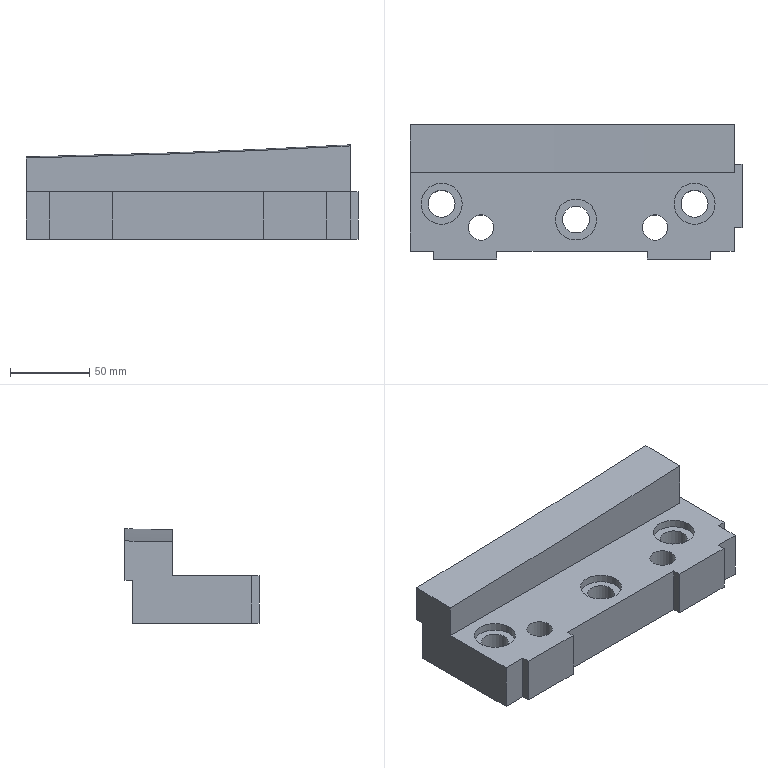Part | NX | features solid 2 | 1 solid | 33 faces | box 210 x 84.909 x 59.687 mm | volume 594644 mm3 | plane 20 | cylinder 8 | spline 5 | commonest cylinder face diameters 17 x3 26 x3 16 x2
STEP:
#1=CARTESIAN_POINT('',(490.,-200.,-40.));
#2=VERTEX_POINT('',#1);
#3=CARTESIAN_POINT('',(490.,-215.,-40.));
#4=VERTEX_POINT('',#3);
#5=CARTESIAN_POINT('',(490.,85.,-40.));
#6=DIRECTION('',(0.,-1.,0.));
#7=VECTOR('',#6,1000.);
#8=LINE('',#5,#7);
#9=EDGE_CURVE('',#2,#4,#8,.T.);
#10=ORIENTED_EDGE('',*,*,#9,.F.);
#11=CARTESIAN_POINT('',(490.,-200.,-10.));
#12=VERTEX_POINT('',#11);
#13=CARTESIAN_POINT('',(490.,-200.,-10.));
#14=DIRECTION('',(0.,0.,-1.));
#15=VECTOR('',#14,1000.);
#16=LINE('',#13,#15);
#17=EDGE_CURVE('',#12,#2,#16,.T.);
#18=ORIENTED_EDGE('',*,*,#17,.F.);
#19=CARTESIAN_POINT('',(490.,-215.,-10.));
#20=VERTEX_POINT('',#19);
#21=CARTESIAN_POINT('',(490.,85.,-10.));
#22=DIRECTION('',(0.,-1.,0.));
#23=VECTOR('',#22,1000.);
#24=LINE('',#21,#23);
#25=EDGE_CURVE('',#12,#20,#24,.T.);
#26=ORIENTED_EDGE('',*,*,#25,.T.);
#27=CARTESIAN_POINT('',(490.,-215.,-10.));
#28=DIRECTION('',(0.,0.,-1.));
#29=VECTOR('',#28,1000.);
#30=LINE('',#27,#29);
#31=EDGE_CURVE('',#20,#4,#30,.T.);
#32=ORIENTED_EDGE('',*,*,#31,.T.);
#33=EDGE_LOOP('',(#10,#18,#26,#32));
#34=FACE_BOUND('',#33,.T.);
#35=CARTESIAN_POINT('',(490.,-135.147,-500.));
#36=DIRECTION('',(-1.,0.00000002,0.));
#37=DIRECTION('',(-0.00000002,-1.,0.));
#38=AXIS2_PLACEMENT_3D('',#35,#36,#37);
#39=PLANE('',#38);
#40=ADVANCED_FACE('',(#34),#39,.F.);
#41=CARTESIAN_POINT('',(435.,-215.,-40.));
#42=VERTEX_POINT('',#41);
#43=CARTESIAN_POINT('',(435.,-215.,-10.));
#44=VERTEX_POINT('',#43);
#45=CARTESIAN_POINT('',(435.,-215.,-40.));
#46=DIRECTION('',(0.,0.,1.));
#47=VECTOR('',#46,1000.);
#48=LINE('',#45,#47);
#49=EDGE_CURVE('',#42,#44,#48,.T.);
#50=ORIENTED_EDGE('',*,*,#49,.T.);
#51=CARTESIAN_POINT('',(340.003,-215.,-10.));
#52=VERTEX_POINT('',#51);
#53=CARTESIAN_POINT('',(660.,-215.,-10.));
#54=DIRECTION('',(1.,0.,0.));
#55=VECTOR('',#54,1000.);
#56=LINE('',#53,#55);
#57=EDGE_CURVE('',#44,#52,#56,.F.);
#58=ORIENTED_EDGE('',*,*,#57,.T.);
#59=CARTESIAN_POINT('',(340.003,-215.,-40.));
#60=VERTEX_POINT('',#59);
#61=CARTESIAN_POINT('',(340.003,-215.,-40.));
#62=DIRECTION('',(0.,0.,1.));
#63=VECTOR('',#62,1000.);
#64=LINE('',#61,#63);
#65=EDGE_CURVE('',#60,#52,#64,.T.);
#66=ORIENTED_EDGE('',*,*,#65,.F.);
#67=CARTESIAN_POINT('',(660.,-215.,-40.));
#68=DIRECTION('',(-1.,0.,0.));
#69=VECTOR('',#68,1000.);
#70=LINE('',#67,#69);
#71=EDGE_CURVE('',#42,#60,#70,.T.);
#72=ORIENTED_EDGE('',*,*,#71,.F.);
#73=EDGE_LOOP('',(#50,#58,#66,#72));
#74=FACE_BOUND('',#73,.T.);
#75=CARTESIAN_POINT('',(660.,-215.,-10.));
#76=DIRECTION('',(0.,-1.,0.));
#77=DIRECTION('',(-1.,0.,0.));
#78=AXIS2_PLACEMENT_3D('',#75,#76,#77);
#79=PLANE('',#78);
#80=ADVANCED_FACE('',(#74),#79,.T.);
#81=CARTESIAN_POINT('',(475.,-215.,-40.));
#82=VERTEX_POINT('',#81);
#83=CARTESIAN_POINT('',(475.,-215.,-10.));
#84=VERTEX_POINT('',#83);
#85=CARTESIAN_POINT('',(475.,-215.,-40.));
#86=DIRECTION('',(0.,0.,1.));
#87=VECTOR('',#86,1000.);
#88=LINE('',#85,#87);
#89=EDGE_CURVE('',#82,#84,#88,.T.);
#90=ORIENTED_EDGE('',*,*,#89,.F.);
#91=CARTESIAN_POINT('',(660.,-215.,-40.));
#92=DIRECTION('',(-1.,0.,0.));
#93=VECTOR('',#92,1000.);
#94=LINE('',#91,#93);
#95=EDGE_CURVE('',#4,#82,#94,.T.);
#96=ORIENTED_EDGE('',*,*,#95,.F.);
#97=ORIENTED_EDGE('',*,*,#31,.F.);
#98=CARTESIAN_POINT('',(660.,-215.,-10.));
#99=DIRECTION('',(1.,0.,0.));
#100=VECTOR('',#99,1000.);
#101=LINE('',#98,#100);
#102=EDGE_CURVE('',#20,#84,#101,.F.);
#103=ORIENTED_EDGE('',*,*,#102,.T.);
#104=EDGE_LOOP('',(#90,#96,#97,#103));
#105=FACE_BOUND('',#104,.T.);
#106=CARTESIAN_POINT('',(660.,-215.,-10.));
#107=DIRECTION('',(0.,-1.,0.));
#108=DIRECTION('',(-1.,0.,0.));
#109=AXIS2_PLACEMENT_3D('',#106,#107,#108);
#110=PLANE('',#109);
#111=ADVANCED_FACE('',(#105),#110,.T.);
#112=CARTESIAN_POINT('',(456.503,-185.,-40.));
#113=VERTEX_POINT('',#112);
#114=CARTESIAN_POINT('',(465.003,-185.,-40.));
#115=DIRECTION('',(0.,0.,-1.));
#116=DIRECTION('',(-1.,0.,0.));
#117=AXIS2_PLACEMENT_3D('',#114,#115,#116);
#118=CIRCLE('',#117,8.5);
#119=EDGE_CURVE('',#113,#113,#118,.F.);
#120=ORIENTED_EDGE('',*,*,#119,.T.);
#121=EDGE_LOOP('',(#120));
#122=FACE_BOUND('',#121,.T.);
#123=CARTESIAN_POINT('',(381.503,-195.,-40.));
#124=VERTEX_POINT('',#123);
#125=CARTESIAN_POINT('',(390.003,-195.,-40.));
#126=DIRECTION('',(0.,0.,-1.));
#127=DIRECTION('',(-1.,0.,0.));
#128=AXIS2_PLACEMENT_3D('',#125,#126,#127);
#129=CIRCLE('',#128,8.5);
#130=EDGE_CURVE('',#124,#124,#129,.F.);
#131=ORIENTED_EDGE('',*,*,#130,.T.);
#132=EDGE_LOOP('',(#131));
#133=FACE_BOUND('',#132,.T.);
#134=CARTESIAN_POINT('',(296.503,-185.,-40.));
#135=VERTEX_POINT('',#134);
#136=CARTESIAN_POINT('',(305.003,-185.,-40.));
#137=DIRECTION('',(0.,0.,-1.));
#138=DIRECTION('',(-1.,0.,0.));
#139=AXIS2_PLACEMENT_3D('',#136,#137,#138);
#140=CIRCLE('',#139,8.5);
#141=EDGE_CURVE('',#135,#135,#140,.F.);
#142=ORIENTED_EDGE('',*,*,#141,.T.);
#143=EDGE_LOOP('',(#142));
#144=FACE_BOUND('',#143,.T.);
#145=CARTESIAN_POINT('',(322.003,-200.,-40.));
#146=VERTEX_POINT('',#145);
#147=CARTESIAN_POINT('',(330.003,-200.,-40.));
#148=DIRECTION('',(0.,0.,-1.));
#149=DIRECTION('',(-1.,0.,0.));
#150=AXIS2_PLACEMENT_3D('',#147,#148,#149);
#151=CIRCLE('',#150,8.);
#152=EDGE_CURVE('',#146,#146,#151,.F.);
#153=ORIENTED_EDGE('',*,*,#152,.T.);
#154=EDGE_LOOP('',(#153));
#155=FACE_BOUND('',#154,.T.);
#156=CARTESIAN_POINT('',(432.003,-200.,-40.));
#157=VERTEX_POINT('',#156);
#158=CARTESIAN_POINT('',(440.003,-200.,-40.));
#159=DIRECTION('',(0.,0.,-1.));
#160=DIRECTION('',(-1.,0.,0.));
#161=AXIS2_PLACEMENT_3D('',#158,#159,#160);
#162=CIRCLE('',#161,8.);
#163=EDGE_CURVE('',#157,#157,#162,.F.);
#164=ORIENTED_EDGE('',*,*,#163,.T.);
#165=EDGE_LOOP('',(#164));
#166=FACE_BOUND('',#165,.T.);
#167=CARTESIAN_POINT('',(490.,-140.147,-40.));
#168=VERTEX_POINT('',#167);
#169=CARTESIAN_POINT('',(490.,-160.,-40.));
#170=VERTEX_POINT('',#169);
#171=CARTESIAN_POINT('',(490.,62.718,-40.));
#172=DIRECTION('',(0.00000002,1.,0.));
#173=VECTOR('',#172,1000.);
#174=LINE('',#171,#173);
#175=EDGE_CURVE('',#168,#170,#174,.F.);
#176=ORIENTED_EDGE('',*,*,#175,.T.);
#177=CARTESIAN_POINT('',(495.,-160.,-40.));
#178=VERTEX_POINT('',#177);
#179=CARTESIAN_POINT('',(490.,-160.,-40.));
#180=DIRECTION('',(1.,0.,0.));
#181=VECTOR('',#180,1000.);
#182=LINE('',#179,#181);
#183=EDGE_CURVE('',#170,#178,#182,.T.);
#184=ORIENTED_EDGE('',*,*,#183,.T.);
#185=CARTESIAN_POINT('',(495.,-200.,-40.));
#186=VERTEX_POINT('',#185);
#187=CARTESIAN_POINT('',(495.,-215.,-40.));
#188=DIRECTION('',(0.,-1.,0.));
#189=VECTOR('',#188,1000.);
#190=LINE('',#187,#189);
#191=EDGE_CURVE('',#178,#186,#190,.T.);
#192=ORIENTED_EDGE('',*,*,#191,.T.);
#193=CARTESIAN_POINT('',(490.,-200.,-40.));
#194=DIRECTION('',(1.,0.,0.));
#195=VECTOR('',#194,1000.);
#196=LINE('',#193,#195);
#197=EDGE_CURVE('',#2,#186,#196,.T.);
#198=ORIENTED_EDGE('',*,*,#197,.F.);
#199=ORIENTED_EDGE('',*,*,#9,.T.);
#200=ORIENTED_EDGE('',*,*,#95,.T.);
#201=CARTESIAN_POINT('',(475.,-220.,-40.));
#202=VERTEX_POINT('',#201);
#203=CARTESIAN_POINT('',(475.,-215.,-40.));
#204=DIRECTION('',(0.,1.,0.));
#205=VECTOR('',#204,1000.);
#206=LINE('',#203,#205);
#207=EDGE_CURVE('',#82,#202,#206,.F.);
#208=ORIENTED_EDGE('',*,*,#207,.T.);
#209=CARTESIAN_POINT('',(435.,-220.,-40.));
#210=VERTEX_POINT('',#209);
#211=CARTESIAN_POINT('',(435.,-220.,-40.));
#212=DIRECTION('',(1.,0.,0.));
#213=VECTOR('',#212,1000.);
#214=LINE('',#211,#213);
#215=EDGE_CURVE('',#210,#202,#214,.T.);
#216=ORIENTED_EDGE('',*,*,#215,.F.);
#217=CARTESIAN_POINT('',(435.,-215.,-40.));
#218=DIRECTION('',(0.,1.,0.));
#219=VECTOR('',#218,1000.);
#220=LINE('',#217,#219);
#221=EDGE_CURVE('',#42,#210,#220,.F.);
#222=ORIENTED_EDGE('',*,*,#221,.F.);
#223=ORIENTED_EDGE('',*,*,#71,.T.);
#224=CARTESIAN_POINT('',(340.003,-220.,-40.));
#225=VERTEX_POINT('',#224);
#226=CARTESIAN_POINT('',(340.003,-215.,-40.));
#227=DIRECTION('',(0.,1.,0.));
#228=VECTOR('',#227,1000.);
#229=LINE('',#226,#228);
#230=EDGE_CURVE('',#60,#225,#229,.F.);
#231=ORIENTED_EDGE('',*,*,#230,.T.);
#232=CARTESIAN_POINT('',(300.003,-220.,-40.));
#233=VERTEX_POINT('',#232);
#234=CARTESIAN_POINT('',(300.003,-220.,-40.));
#235=DIRECTION('',(1.,0.,0.));
#236=VECTOR('',#235,1000.);
#237=LINE('',#234,#236);
#238=EDGE_CURVE('',#233,#225,#237,.T.);
#239=ORIENTED_EDGE('',*,*,#238,.F.);
#240=CARTESIAN_POINT('',(300.003,-215.,-40.));
#241=VERTEX_POINT('',#240);
#242=CARTESIAN_POINT('',(300.003,-215.,-40.));
#243=DIRECTION('',(0.,1.,0.));
#244=VECTOR('',#243,1000.);
#245=LINE('',#242,#244);
#246=EDGE_CURVE('',#241,#233,#245,.F.);
#247=ORIENTED_EDGE('',*,*,#246,.F.);
#248=CARTESIAN_POINT('',(285.003,-215.,-40.));
#249=VERTEX_POINT('',#248);
#250=CARTESIAN_POINT('',(660.,-215.,-40.));
#251=DIRECTION('',(-1.,0.,0.));
#252=VECTOR('',#251,1000.);
#253=LINE('',#250,#252);
#254=EDGE_CURVE('',#241,#249,#253,.T.);
#255=ORIENTED_EDGE('',*,*,#254,.T.);
#256=CARTESIAN_POINT('',(285.,-140.12,-40.));
#257=VERTEX_POINT('',#256);
#258=CARTESIAN_POINT('',(284.994,62.719,-40.));
#259=DIRECTION('',(-0.00003252,1.,0.));
#260=VECTOR('',#259,1000.);
#261=LINE('',#258,#260);
#262=EDGE_CURVE('',#257,#249,#261,.F.);
#263=ORIENTED_EDGE('',*,*,#262,.F.);
#264=CARTESIAN_POINT('',(285.,-140.12,-40.));
#265=CARTESIAN_POINT('',(319.167,-140.081,-40.));
#266=CARTESIAN_POINT('',(387.5,-140.101,-40.));
#267=CARTESIAN_POINT('',(455.833,-140.101,-40.));
#268=CARTESIAN_POINT('',(490.,-140.147,-40.));
#269=B_SPLINE_CURVE_WITH_KNOTS('',3,(#264,#265,#266,#267,#268),.UNSPECIFIED.,.F.,.F.,(4,1,4),(0.00123,0.1037,0.2062),.UNSPECIFIED.);
#270=EDGE_CURVE('',#257,#168,#269,.T.);
#271=ORIENTED_EDGE('',*,*,#270,.T.);
#272=EDGE_LOOP('',(#176,#184,#192,#198,#199,#200,#208,#216,#222,#223,#231,#239,#247,#255,#263,#271));
#273=FACE_BOUND('',#272,.T.);
#274=CARTESIAN_POINT('',(248.595,62.718,-40.));
#275=DIRECTION('',(0.,0.,-1.));
#276=DIRECTION('',(1.,0.,0.));
#277=AXIS2_PLACEMENT_3D('',#274,#275,#276);
#278=PLANE('',#277);
#279=ADVANCED_FACE('',(#122,#133,#144,#155,#166,#273),#278,.T.);
#280=CARTESIAN_POINT('',(490.,-135.147,-5.35));
#281=VERTEX_POINT('',#280);
#282=CARTESIAN_POINT('',(490.,-135.147,19.687));
#283=VERTEX_POINT('',#282);
#284=CARTESIAN_POINT('',(490.,-135.147,-500.));
#285=DIRECTION('',(0.,0.,1.));
#286=VECTOR('',#285,1000.);
#287=LINE('',#284,#286);
#288=EDGE_CURVE('',#281,#283,#287,.T.);
#289=ORIENTED_EDGE('',*,*,#288,.F.);
#290=CARTESIAN_POINT('',(285.,-135.12,-12.944));
#291=VERTEX_POINT('',#290);
#292=CARTESIAN_POINT('',(490.,-135.147,-5.35));
#293=CARTESIAN_POINT('',(455.858,-135.101,-7.199));
#294=CARTESIAN_POINT('',(404.622,-135.095,-9.527));
#295=CARTESIAN_POINT('',(344.818,-135.095,-11.511));
#296=CARTESIAN_POINT('',(310.638,-135.1,-12.377));
#297=CARTESIAN_POINT('',(293.547,-135.11,-12.83));
#298=CARTESIAN_POINT('',(285.,-135.12,-12.944));
#299=B_SPLINE_CURVE_WITH_KNOTS('',3,(#292,#293,#294,#295,#296,#297,#298),.UNSPECIFIED.,.F.,.F.,(4,1,1,1,4),(0.,0.1026,0.1539,0.1795,0.2052),.UNSPECIFIED.);
#300=EDGE_CURVE('',#281,#291,#299,.T.);
#301=ORIENTED_EDGE('',*,*,#300,.T.);
#302=CARTESIAN_POINT('',(285.,-135.12,12.056));
#303=VERTEX_POINT('',#302);
#304=CARTESIAN_POINT('',(285.,-135.12,-500.));
#305=DIRECTION('',(0.,0.,1.));
#306=VECTOR('',#305,1000.);
#307=LINE('',#304,#306);
#308=EDGE_CURVE('',#291,#303,#307,.T.);
#309=ORIENTED_EDGE('',*,*,#308,.T.);
#310=CARTESIAN_POINT('',(285.,-135.12,12.056));
#311=CARTESIAN_POINT('',(319.186,-135.081,12.742));
#312=CARTESIAN_POINT('',(387.542,-135.101,14.7));
#313=CARTESIAN_POINT('',(455.858,-135.101,17.83));
#314=CARTESIAN_POINT('',(490.,-135.147,19.687));
#315=B_SPLINE_CURVE_WITH_KNOTS('',3,(#310,#311,#312,#313,#314),.UNSPECIFIED.,.F.,.F.,(4,1,4),(0.,0.1026,0.2051),.UNSPECIFIED.);
#316=EDGE_CURVE('',#303,#283,#315,.T.);
#317=ORIENTED_EDGE('',*,*,#316,.T.);
#318=EDGE_LOOP('',(#289,#301,#309,#317));
#319=FACE_BOUND('',#318,.T.);
#320=CARTESIAN_POINT('',(285.,-135.12,-13.14));
#321=CARTESIAN_POINT('',(285.,-135.12,19.883));
#322=CARTESIAN_POINT('',(319.184,-135.081,-13.14));
#323=CARTESIAN_POINT('',(319.184,-135.081,19.883));
#324=CARTESIAN_POINT('',(387.544,-135.101,-13.14));
#325=CARTESIAN_POINT('',(387.544,-135.101,19.883));
#326=CARTESIAN_POINT('',(455.858,-135.101,-13.14));
#327=CARTESIAN_POINT('',(455.858,-135.101,19.883));
#328=CARTESIAN_POINT('',(490.,-135.147,-13.14));
#329=CARTESIAN_POINT('',(490.,-135.147,19.883));
#330=B_SPLINE_SURFACE_WITH_KNOTS('',3,1,((#320,#321),(#322,#323),(#324,#325),(#326,#327),(#328,#329)),.SURF_OF_LINEAR_EXTRUSION.,.F.,.F.,.F.,(4,1,4),(2,2),(0.,0.5,1.),(0.,1.),.UNSPECIFIED.);
#331=ADVANCED_FACE('',(#319),#330,.F.);
#332=CARTESIAN_POINT('',(490.,-165.147,-10.));
#333=VERTEX_POINT('',#332);
#334=CARTESIAN_POINT('',(490.,-165.147,18.99));
#335=VERTEX_POINT('',#334);
#336=CARTESIAN_POINT('',(490.,-165.147,-500.));
#337=DIRECTION('',(0.,0.,1.));
#338=VECTOR('',#337,1000.);
#339=LINE('',#336,#338);
#340=EDGE_CURVE('',#333,#335,#339,.T.);
#341=ORIENTED_EDGE('',*,*,#340,.F.);
#342=CARTESIAN_POINT('',(490.,-160.,-10.));
#343=VERTEX_POINT('',#342);
#344=CARTESIAN_POINT('',(490.,-215.,-10.));
#345=DIRECTION('',(0.,-1.,0.));
#346=VECTOR('',#345,1000.);
#347=LINE('',#344,#346);
#348=EDGE_CURVE('',#343,#333,#347,.T.);
#349=ORIENTED_EDGE('',*,*,#348,.F.);
#350=CARTESIAN_POINT('',(490.,-160.,-10.));
#351=DIRECTION('',(0.,0.,-1.));
#352=VECTOR('',#351,1000.);
#353=LINE('',#350,#352);
#354=EDGE_CURVE('',#343,#170,#353,.T.);
#355=ORIENTED_EDGE('',*,*,#354,.T.);
#356=ORIENTED_EDGE('',*,*,#175,.F.);
#357=CARTESIAN_POINT('',(490.,-140.147,-5.35));
#358=VERTEX_POINT('',#357);
#359=CARTESIAN_POINT('',(490.,-140.147,-155.35));
#360=DIRECTION('',(0.,0.,-1.));
#361=VECTOR('',#360,1000.);
#362=LINE('',#359,#361);
#363=EDGE_CURVE('',#168,#358,#362,.F.);
#364=ORIENTED_EDGE('',*,*,#363,.T.);
#365=CARTESIAN_POINT('',(490.,-140.147,-5.35));
#366=CARTESIAN_POINT('',(490.,-138.48,-5.35));
#367=CARTESIAN_POINT('',(490.,-136.814,-5.35));
#368=CARTESIAN_POINT('',(490.,-135.147,-5.35));
#369=B_SPLINE_CURVE_WITH_KNOTS('',3,(#365,#366,#367,#368),.UNSPECIFIED.,.F.,.F.,(4,4),(0.,0.005),.UNSPECIFIED.);
#370=EDGE_CURVE('',#358,#281,#369,.T.);
#371=ORIENTED_EDGE('',*,*,#370,.T.);
#372=ORIENTED_EDGE('',*,*,#288,.T.);
#373=CARTESIAN_POINT('',(490.,-135.147,19.687));
#374=CARTESIAN_POINT('',(490.,-145.147,19.455));
#375=CARTESIAN_POINT('',(490.,-155.147,19.222));
#376=CARTESIAN_POINT('',(490.,-165.147,18.99));
#377=B_SPLINE_CURVE_WITH_KNOTS('',3,(#373,#374,#375,#376),.UNSPECIFIED.,.F.,.F.,(4,4),(0.,0.03001),.UNSPECIFIED.);
#378=EDGE_CURVE('',#283,#335,#377,.T.);
#379=ORIENTED_EDGE('',*,*,#378,.T.);
#380=EDGE_LOOP('',(#341,#349,#355,#356,#364,#371,#372,#379));
#381=FACE_BOUND('',#380,.T.);
#382=CARTESIAN_POINT('',(490.,-135.147,-500.));
#383=DIRECTION('',(-1.,0.00000002,0.));
#384=DIRECTION('',(-0.00000002,-1.,0.));
#385=AXIS2_PLACEMENT_3D('',#382,#383,#384);
#386=PLANE('',#385);
#387=ADVANCED_FACE('',(#381),#386,.F.);
#388=CARTESIAN_POINT('',(285.001,-165.12,-10.));
#389=VERTEX_POINT('',#388);
#390=CARTESIAN_POINT('',(285.001,-165.12,-10.));
#391=CARTESIAN_POINT('',(319.155,-165.081,-10.));
#392=CARTESIAN_POINT('',(387.552,-165.101,-10.));
#393=CARTESIAN_POINT('',(455.871,-165.101,-10.));
#394=CARTESIAN_POINT('',(490.,-165.147,-10.));
#395=B_SPLINE_CURVE_WITH_KNOTS('',3,(#390,#391,#392,#393,#394),.UNSPECIFIED.,.F.,.F.,(4,1,4),(0.,0.5,1.),.UNSPECIFIED.);
#396=EDGE_CURVE('',#333,#389,#395,.F.);
#397=ORIENTED_EDGE('',*,*,#396,.F.);
#398=ORIENTED_EDGE('',*,*,#340,.T.);
#399=CARTESIAN_POINT('',(285.001,-165.12,11.359));
#400=VERTEX_POINT('',#399);
#401=CARTESIAN_POINT('',(285.001,-165.12,11.359));
#402=CARTESIAN_POINT('',(319.186,-165.081,12.046));
#403=CARTESIAN_POINT('',(387.546,-165.101,14.004));
#404=CARTESIAN_POINT('',(455.858,-165.101,17.134));
#405=CARTESIAN_POINT('',(490.,-165.147,18.99));
#406=B_SPLINE_CURVE_WITH_KNOTS('',3,(#401,#402,#403,#404,#405),.UNSPECIFIED.,.F.,.F.,(4,1,4),(0.,0.1026,0.2052),.UNSPECIFIED.);
#407=EDGE_CURVE('',#400,#335,#406,.T.);
#408=ORIENTED_EDGE('',*,*,#407,.F.);
#409=CARTESIAN_POINT('',(285.001,-165.12,-500.));
#410=DIRECTION('',(0.,0.,1.));
#411=VECTOR('',#410,1000.);
#412=LINE('',#409,#411);
#413=EDGE_CURVE('',#389,#400,#412,.T.);
#414=ORIENTED_EDGE('',*,*,#413,.F.);
#415=EDGE_LOOP('',(#397,#398,#408,#414));
#416=FACE_BOUND('',#415,.T.);
#417=CARTESIAN_POINT('',(285.001,-165.12,-10.));
#418=CARTESIAN_POINT('',(285.001,-165.12,19.164));
#419=CARTESIAN_POINT('',(319.157,-165.081,-10.));
#420=CARTESIAN_POINT('',(319.157,-165.081,19.164));
#421=CARTESIAN_POINT('',(387.554,-165.101,-10.));
#422=CARTESIAN_POINT('',(387.554,-165.101,19.164));
#423=CARTESIAN_POINT('',(455.872,-165.101,-10.));
#424=CARTESIAN_POINT('',(455.872,-165.101,19.164));
#425=CARTESIAN_POINT('',(490.,-165.147,-10.));
#426=CARTESIAN_POINT('',(490.,-165.147,19.164));
#427=B_SPLINE_SURFACE_WITH_KNOTS('',3,1,((#417,#418),(#419,#420),(#421,#422),(#423,#424),(#425,#426)),.SURF_OF_LINEAR_EXTRUSION.,.F.,.F.,.F.,(4,1,4),(2,2),(0.,0.5,1.),(0.,1.),.UNSPECIFIED.);
#428=ADVANCED_FACE('',(#416),#427,.T.);
#429=CARTESIAN_POINT('',(285.003,-215.,-10.));
#430=VERTEX_POINT('',#429);
#431=CARTESIAN_POINT('',(285.,-135.12,-10.));
#432=DIRECTION('',(-0.00003252,1.,0.));
#433=VECTOR('',#432,1000.);
#434=LINE('',#431,#433);
#435=EDGE_CURVE('',#389,#430,#434,.F.);
#436=ORIENTED_EDGE('',*,*,#435,.F.);
#437=ORIENTED_EDGE('',*,*,#413,.T.);
#438=CARTESIAN_POINT('',(285.,-135.12,12.056));
#439=CARTESIAN_POINT('',(285.,-145.12,11.823));
#440=CARTESIAN_POINT('',(285.001,-155.12,11.591));
#441=CARTESIAN_POINT('',(285.001,-165.12,11.359));
#442=B_SPLINE_CURVE_WITH_KNOTS('',3,(#438,#439,#440,#441),.UNSPECIFIED.,.F.,.F.,(4,4),(0.,0.03001),.UNSPECIFIED.);
#443=EDGE_CURVE('',#303,#400,#442,.T.);
#444=ORIENTED_EDGE('',*,*,#443,.F.);
#445=ORIENTED_EDGE('',*,*,#308,.F.);
#446=CARTESIAN_POINT('',(285.,-140.12,-12.945));
#447=VERTEX_POINT('',#446);
#448=CARTESIAN_POINT('',(285.,-140.12,-12.945));
#449=CARTESIAN_POINT('',(285.,-138.453,-12.945));
#450=CARTESIAN_POINT('',(285.,-136.787,-12.945));
#451=CARTESIAN_POINT('',(285.,-135.12,-12.944));
#452=B_SPLINE_CURVE_WITH_KNOTS('',3,(#448,#449,#450,#451),.UNSPECIFIED.,.F.,.F.,(4,4),(0.,0.005),.UNSPECIFIED.);
#453=EDGE_CURVE('',#447,#291,#452,.T.);
#454=ORIENTED_EDGE('',*,*,#453,.F.);
#455=CARTESIAN_POINT('',(285.,-140.12,-162.945));
#456=DIRECTION('',(0.,0.,-1.));
#457=VECTOR('',#456,1000.);
#458=LINE('',#455,#457);
#459=EDGE_CURVE('',#257,#447,#458,.F.);
#460=ORIENTED_EDGE('',*,*,#459,.F.);
#461=ORIENTED_EDGE('',*,*,#262,.T.);
#462=CARTESIAN_POINT('',(285.003,-215.,-500.));
#463=DIRECTION('',(0.,0.,1.));
#464=VECTOR('',#463,1000.);
#465=LINE('',#462,#464);
#466=EDGE_CURVE('',#249,#430,#465,.T.);
#467=ORIENTED_EDGE('',*,*,#466,.T.);
#468=EDGE_LOOP('',(#436,#437,#444,#445,#454,#460,#461,#467));
#469=FACE_BOUND('',#468,.T.);
#470=CARTESIAN_POINT('',(285.,-135.12,-500.));
#471=DIRECTION('',(-1.,-0.00003252,0.));
#472=DIRECTION('',(0.00003252,-1.,0.));
#473=AXIS2_PLACEMENT_3D('',#470,#471,#472);
#474=PLANE('',#473);
#475=ADVANCED_FACE('',(#469),#474,.T.);
#476=ORIENTED_EDGE('',*,*,#443,.T.);
#477=ORIENTED_EDGE('',*,*,#407,.T.);
#478=ORIENTED_EDGE('',*,*,#378,.F.);
#479=ORIENTED_EDGE('',*,*,#316,.F.);
#480=EDGE_LOOP('',(#476,#477,#478,#479));
#481=FACE_BOUND('',#480,.T.);
#482=CARTESIAN_POINT('',(490.,-134.964,19.691));
#483=CARTESIAN_POINT('',(490.,-165.478,18.983));
#484=CARTESIAN_POINT('',(421.297,-134.878,15.955));
#485=CARTESIAN_POINT('',(421.297,-165.391,15.246));
#486=CARTESIAN_POINT('',(352.547,-134.819,13.404));
#487=CARTESIAN_POINT('',(352.547,-165.332,12.695));
#488=CARTESIAN_POINT('',(283.77,-134.787,12.039));
#489=CARTESIAN_POINT('',(283.77,-165.3,11.33));
#490=(BOUNDED_SURFACE()B_SPLINE_SURFACE(3,1,((#482,#483),(#484,#485),(#486,#487),(#488,#489)),.SURF_OF_LINEAR_EXTRUSION.,.F.,.F.,.F.)B_SPLINE_SURFACE_WITH_KNOTS((4,4),(2,2),(0.2652,0.4659),(0.6408,0.6712),.PIECEWISE_BEZIER_KNOTS.)GEOMETRIC_REPRESENTATION_ITEM()RATIONAL_B_SPLINE_SURFACE(((0.9999,0.9999),(1.,1.),(1.,1.),(1.,1.)))REPRESENTATION_ITEM('')SURFACE());
#491=ADVANCED_FACE('',(#481),#490,.T.);
#492=CARTESIAN_POINT('',(285.,-140.12,-12.945));
#493=CARTESIAN_POINT('',(293.547,-140.11,-12.831));
#494=CARTESIAN_POINT('',(310.636,-140.097,-12.377));
#495=CARTESIAN_POINT('',(344.816,-140.088,-11.511));
#496=CARTESIAN_POINT('',(404.623,-140.101,-9.527));
#497=CARTESIAN_POINT('',(455.861,-140.101,-7.199));
#498=CARTESIAN_POINT('',(490.,-140.147,-5.35));
#499=B_SPLINE_CURVE_WITH_KNOTS('',3,(#492,#493,#494,#495,#496,#497,#498),.UNSPECIFIED.,.F.,.F.,(4,1,1,1,4),(-0.00002676,0.125,0.25,0.5,1.),.UNSPECIFIED.);
#500=EDGE_CURVE('',#358,#447,#499,.F.);
#501=ORIENTED_EDGE('',*,*,#500,.T.);
#502=ORIENTED_EDGE('',*,*,#453,.T.);
#503=ORIENTED_EDGE('',*,*,#300,.F.);
#504=ORIENTED_EDGE('',*,*,#370,.F.);
#505=EDGE_LOOP('',(#501,#502,#503,#504));
#506=FACE_BOUND('',#505,.T.);
#507=CARTESIAN_POINT('',(491.229,-140.149,-5.283));
#508=CARTESIAN_POINT('',(490.817,-140.148,-5.305));
#509=CARTESIAN_POINT('',(490.405,-140.148,-5.328));
#510=CARTESIAN_POINT('',(489.993,-140.147,-5.35));
#511=CARTESIAN_POINT('',(455.856,-140.101,-7.199));
#512=CARTESIAN_POINT('',(421.701,-140.101,-8.758));
#513=CARTESIAN_POINT('',(370.447,-140.093,-10.657));
#514=CARTESIAN_POINT('',(353.361,-140.09,-11.218));
#515=CARTESIAN_POINT('',(327.729,-140.093,-11.949));
#516=CARTESIAN_POINT('',(319.185,-140.095,-12.175));
#517=CARTESIAN_POINT('',(306.368,-140.102,-12.486));
#518=CARTESIAN_POINT('',(302.096,-140.104,-12.585));
#519=CARTESIAN_POINT('',(293.551,-140.111,-12.774));
#520=CARTESIAN_POINT('',(289.279,-140.115,-12.887));
#521=CARTESIAN_POINT('',(285.006,-140.12,-12.944));
#522=CARTESIAN_POINT('',(284.594,-140.121,-12.95));
#523=CARTESIAN_POINT('',(284.182,-140.121,-12.955));
#524=CARTESIAN_POINT('',(283.769,-140.121,-12.961));
#525=CARTESIAN_POINT('',(491.236,-135.118,-5.283));
#526=CARTESIAN_POINT('',(490.824,-135.117,-5.305));
#527=CARTESIAN_POINT('',(490.412,-135.117,-5.328));
#528=CARTESIAN_POINT('',(490.,-135.116,-5.35));
#529=CARTESIAN_POINT('',(455.858,-135.07,-7.199));
#530=CARTESIAN_POINT('',(421.701,-135.07,-8.758));
#531=CARTESIAN_POINT('',(370.448,-135.063,-10.657));
#532=CARTESIAN_POINT('',(353.361,-135.059,-11.218));
#533=CARTESIAN_POINT('',(327.728,-135.062,-11.949));
#534=CARTESIAN_POINT('',(319.183,-135.064,-12.175));
#535=CARTESIAN_POINT('',(306.365,-135.071,-12.486));
#536=CARTESIAN_POINT('',(302.092,-135.073,-12.585));
#537=CARTESIAN_POINT('',(293.546,-135.08,-12.774));
#538=CARTESIAN_POINT('',(289.274,-135.084,-12.887));
#539=CARTESIAN_POINT('',(285.,-135.089,-12.944));
#540=CARTESIAN_POINT('',(284.588,-135.09,-12.95));
#541=CARTESIAN_POINT('',(284.176,-135.09,-12.955));
#542=CARTESIAN_POINT('',(283.764,-135.091,-12.961));
#543=B_SPLINE_SURFACE_WITH_KNOTS('',1,3,((#507,#508,#509,#510,#511,#512,#513,#514,#515,#516,#517,#518,#519,#520,#521,#522,#523,#524),(#525,#526,#527,#528,#529,#530,#531,#532,#533,#534,#535,#536,#537,#538,#539,#540,#541,#542)),.RULED_SURF.,.F.,.F.,.F.,(2,2),(4,3,2,2,2,2,3,4),(0.,0.5031),(-0.006033,0.,0.5,0.75,0.875,0.9375,1.,1.006),.UNSPECIFIED.);
#544=ADVANCED_FACE('',(#506),#543,.F.);
#545=ORIENTED_EDGE('',*,*,#270,.F.);
#546=ORIENTED_EDGE('',*,*,#459,.T.);
#547=ORIENTED_EDGE('',*,*,#500,.F.);
#548=ORIENTED_EDGE('',*,*,#363,.F.);
#549=EDGE_LOOP('',(#545,#546,#547,#548));
#550=FACE_BOUND('',#549,.T.);
#551=CARTESIAN_POINT('',(490.,-140.147,-5.35));
#552=CARTESIAN_POINT('',(490.,-140.147,-40.208));
#553=CARTESIAN_POINT('',(455.856,-140.101,-7.199));
#554=CARTESIAN_POINT('',(455.856,-140.101,-42.057));
#555=CARTESIAN_POINT('',(404.624,-140.101,-9.527));
#556=CARTESIAN_POINT('',(404.624,-140.101,-44.385));
#557=CARTESIAN_POINT('',(344.816,-140.088,-11.511));
#558=CARTESIAN_POINT('',(344.816,-140.088,-46.37));
#559=CARTESIAN_POINT('',(310.636,-140.097,-12.377));
#560=CARTESIAN_POINT('',(310.636,-140.097,-47.235));
#561=CARTESIAN_POINT('',(293.548,-140.11,-12.831));
#562=CARTESIAN_POINT('',(293.548,-140.11,-47.689));
#563=CARTESIAN_POINT('',(285.,-140.12,-12.945));
#564=CARTESIAN_POINT('',(285.,-140.12,-47.803));
#565=B_SPLINE_SURFACE_WITH_KNOTS('',3,1,((#551,#552),(#553,#554),(#555,#556),(#557,#558),(#559,#560),(#561,#562),(#563,#564)),.SURF_OF_LINEAR_EXTRUSION.,.F.,.F.,.F.,(4,1,1,1,4),(2,2),(-0.00003311,0.5,0.75,0.875,1.),(0.,1.),.UNSPECIFIED.);
#566=ADVANCED_FACE('',(#550),#565,.F.);
#567=CARTESIAN_POINT('',(478.003,-185.,-10.));
#568=VERTEX_POINT('',#567);
#569=CARTESIAN_POINT('',(465.003,-185.,-10.));
#570=DIRECTION('',(0.,0.,1.));
#571=DIRECTION('',(1.,0.,0.));
#572=AXIS2_PLACEMENT_3D('',#569,#570,#571);
#573=CIRCLE('',#572,13.);
#574=EDGE_CURVE('',#568,#568,#573,.T.);
#575=ORIENTED_EDGE('',*,*,#574,.F.);
#576=EDGE_LOOP('',(#575));
#577=FACE_BOUND('',#576,.T.);
#578=CARTESIAN_POINT('',(403.003,-195.,-10.));
#579=VERTEX_POINT('',#578);
#580=CARTESIAN_POINT('',(390.003,-195.,-10.));
#581=DIRECTION('',(0.,0.,1.));
#582=DIRECTION('',(1.,0.,0.));
#583=AXIS2_PLACEMENT_3D('',#580,#581,#582);
#584=CIRCLE('',#583,13.);
#585=EDGE_CURVE('',#579,#579,#584,.T.);
#586=ORIENTED_EDGE('',*,*,#585,.F.);
#587=EDGE_LOOP('',(#586));
#588=FACE_BOUND('',#587,.T.);
#589=CARTESIAN_POINT('',(318.003,-185.,-10.));
#590=VERTEX_POINT('',#589);
#591=CARTESIAN_POINT('',(305.003,-185.,-10.));
#592=DIRECTION('',(0.,0.,1.));
#593=DIRECTION('',(1.,0.,0.));
#594=AXIS2_PLACEMENT_3D('',#591,#592,#593);
#595=CIRCLE('',#594,13.);
#596=EDGE_CURVE('',#590,#590,#595,.T.);
#597=ORIENTED_EDGE('',*,*,#596,.F.);
#598=EDGE_LOOP('',(#597));
#599=FACE_BOUND('',#598,.T.);
#600=CARTESIAN_POINT('',(338.003,-200.,-10.));
#601=VERTEX_POINT('',#600);
#602=CARTESIAN_POINT('',(330.003,-200.,-10.));
#603=DIRECTION('',(0.,0.,1.));
#604=DIRECTION('',(1.,0.,0.));
#605=AXIS2_PLACEMENT_3D('',#602,#603,#604);
#606=CIRCLE('',#605,8.);
#607=EDGE_CURVE('',#601,#601,#606,.T.);
#608=ORIENTED_EDGE('',*,*,#607,.F.);
#609=EDGE_LOOP('',(#608));
#610=FACE_BOUND('',#609,.T.);
#611=CARTESIAN_POINT('',(448.003,-200.,-10.));
#612=VERTEX_POINT('',#611);
#613=CARTESIAN_POINT('',(440.003,-200.,-10.));
#614=DIRECTION('',(0.,0.,1.));
#615=DIRECTION('',(1.,0.,0.));
#616=AXIS2_PLACEMENT_3D('',#613,#614,#615);
#617=CIRCLE('',#616,8.);
#618=EDGE_CURVE('',#612,#612,#617,.T.);
#619=ORIENTED_EDGE('',*,*,#618,.F.);
#620=EDGE_LOOP('',(#619));
#621=FACE_BOUND('',#620,.T.);
#622=ORIENTED_EDGE('',*,*,#25,.F.);
#623=CARTESIAN_POINT('',(495.,-200.,-10.));
#624=VERTEX_POINT('',#623);
#625=CARTESIAN_POINT('',(490.,-200.,-10.));
#626=DIRECTION('',(1.,0.,0.));
#627=VECTOR('',#626,1000.);
#628=LINE('',#625,#627);
#629=EDGE_CURVE('',#12,#624,#628,.T.);
#630=ORIENTED_EDGE('',*,*,#629,.T.);
#631=CARTESIAN_POINT('',(495.,-160.,-10.));
#632=VERTEX_POINT('',#631);
#633=CARTESIAN_POINT('',(495.,-215.,-10.));
#634=DIRECTION('',(0.,-1.,0.));
#635=VECTOR('',#634,1000.);
#636=LINE('',#633,#635);
#637=EDGE_CURVE('',#632,#624,#636,.T.);
#638=ORIENTED_EDGE('',*,*,#637,.F.);
#639=CARTESIAN_POINT('',(490.,-160.,-10.));
#640=DIRECTION('',(-1.,0.,0.));
#641=VECTOR('',#640,1000.);
#642=LINE('',#639,#641);
#643=EDGE_CURVE('',#343,#632,#642,.F.);
#644=ORIENTED_EDGE('',*,*,#643,.F.);
#645=ORIENTED_EDGE('',*,*,#348,.T.);
#646=ORIENTED_EDGE('',*,*,#396,.T.);
#647=ORIENTED_EDGE('',*,*,#435,.T.);
#648=CARTESIAN_POINT('',(300.003,-215.,-10.));
#649=VERTEX_POINT('',#648);
#650=CARTESIAN_POINT('',(660.,-215.,-10.));
#651=DIRECTION('',(1.,0.,0.));
#652=VECTOR('',#651,1000.);
#653=LINE('',#650,#652);
#654=EDGE_CURVE('',#649,#430,#653,.F.);
#655=ORIENTED_EDGE('',*,*,#654,.F.);
#656=CARTESIAN_POINT('',(300.003,-220.,-10.));
#657=VERTEX_POINT('',#656);
#658=CARTESIAN_POINT('',(300.003,-215.,-10.));
#659=DIRECTION('',(0.,1.,0.));
#660=VECTOR('',#659,1000.);
#661=LINE('',#658,#660);
#662=EDGE_CURVE('',#649,#657,#661,.F.);
#663=ORIENTED_EDGE('',*,*,#662,.T.);
#664=CARTESIAN_POINT('',(340.003,-220.,-10.));
#665=VERTEX_POINT('',#664);
#666=CARTESIAN_POINT('',(300.003,-220.,-10.));
#667=DIRECTION('',(1.,0.,0.));
#668=VECTOR('',#667,1000.);
#669=LINE('',#666,#668);
#670=EDGE_CURVE('',#657,#665,#669,.T.);
#671=ORIENTED_EDGE('',*,*,#670,.T.);
#672=CARTESIAN_POINT('',(340.003,-215.,-10.));
#673=DIRECTION('',(0.,1.,0.));
#674=VECTOR('',#673,1000.);
#675=LINE('',#672,#674);
#676=EDGE_CURVE('',#52,#665,#675,.F.);
#677=ORIENTED_EDGE('',*,*,#676,.F.);
#678=ORIENTED_EDGE('',*,*,#57,.F.);
#679=CARTESIAN_POINT('',(435.,-220.,-10.));
#680=VERTEX_POINT('',#679);
#681=CARTESIAN_POINT('',(435.,-215.,-10.));
#682=DIRECTION('',(0.,1.,0.));
#683=VECTOR('',#682,1000.);
#684=LINE('',#681,#683);
#685=EDGE_CURVE('',#44,#680,#684,.F.);
#686=ORIENTED_EDGE('',*,*,#685,.T.);
#687=CARTESIAN_POINT('',(475.,-220.,-10.));
#688=VERTEX_POINT('',#687);
#689=CARTESIAN_POINT('',(435.,-220.,-10.));
#690=DIRECTION('',(1.,0.,0.));
#691=VECTOR('',#690,1000.);
#692=LINE('',#689,#691);
#693=EDGE_CURVE('',#680,#688,#692,.T.);
#694=ORIENTED_EDGE('',*,*,#693,.T.);
#695=CARTESIAN_POINT('',(475.,-215.,-10.));
#696=DIRECTION('',(0.,1.,0.));
#697=VECTOR('',#696,1000.);
#698=LINE('',#695,#697);
#699=EDGE_CURVE('',#84,#688,#698,.F.);
#700=ORIENTED_EDGE('',*,*,#699,.F.);
#701=ORIENTED_EDGE('',*,*,#102,.F.);
#702=EDGE_LOOP('',(#622,#630,#638,#644,#645,#646,#647,#655,#663,#671,#677,#678,#686,#694,#700,#701));
#703=FACE_BOUND('',#702,.T.);
#704=CARTESIAN_POINT('',(660.,85.,-10.));
#705=DIRECTION('',(0.,0.,1.));
#706=DIRECTION('',(1.,0.,0.));
#707=AXIS2_PLACEMENT_3D('',#704,#705,#706);
#708=PLANE('',#707);
#709=ADVANCED_FACE('',(#577,#588,#599,#610,#621,#703),#708,.T.);
#710=ORIENTED_EDGE('',*,*,#254,.F.);
#711=CARTESIAN_POINT('',(300.003,-215.,-40.));
#712=DIRECTION('',(0.,0.,1.));
#713=VECTOR('',#712,1000.);
#714=LINE('',#711,#713);
#715=EDGE_CURVE('',#241,#649,#714,.T.);
#716=ORIENTED_EDGE('',*,*,#715,.T.);
#717=ORIENTED_EDGE('',*,*,#654,.T.);
#718=ORIENTED_EDGE('',*,*,#466,.F.);
#719=EDGE_LOOP('',(#710,#716,#717,#718));
#720=FACE_BOUND('',#719,.T.);
#721=CARTESIAN_POINT('',(660.,-215.,-10.));
#722=DIRECTION('',(0.,-1.,0.));
#723=DIRECTION('',(-1.,0.,0.));
#724=AXIS2_PLACEMENT_3D('',#721,#722,#723);
#725=PLANE('',#724);
#726=ADVANCED_FACE('',(#720),#725,.T.);
#727=ORIENTED_EDGE('',*,*,#246,.T.);
#728=CARTESIAN_POINT('',(300.003,-220.,-40.));
#729=DIRECTION('',(0.,0.,1.));
#730=VECTOR('',#729,1000.);
#731=LINE('',#728,#730);
#732=EDGE_CURVE('',#233,#657,#731,.T.);
#733=ORIENTED_EDGE('',*,*,#732,.T.);
#734=ORIENTED_EDGE('',*,*,#662,.F.);
#735=ORIENTED_EDGE('',*,*,#715,.F.);
#736=EDGE_LOOP('',(#727,#733,#734,#735));
#737=FACE_BOUND('',#736,.T.);
#738=CARTESIAN_POINT('',(300.003,-215.,-40.));
#739=DIRECTION('',(-1.,0.,0.));
#740=DIRECTION('',(0.,0.,1.));
#741=AXIS2_PLACEMENT_3D('',#738,#739,#740);
#742=PLANE('',#741);
#743=ADVANCED_FACE('',(#737),#742,.T.);
#744=ORIENTED_EDGE('',*,*,#676,.T.);
#745=CARTESIAN_POINT('',(340.003,-220.,-40.));
#746=DIRECTION('',(0.,0.,1.));
#747=VECTOR('',#746,1000.);
#748=LINE('',#745,#747);
#749=EDGE_CURVE('',#225,#665,#748,.T.);
#750=ORIENTED_EDGE('',*,*,#749,.F.);
#751=ORIENTED_EDGE('',*,*,#230,.F.);
#752=ORIENTED_EDGE('',*,*,#65,.T.);
#753=EDGE_LOOP('',(#744,#750,#751,#752));
#754=FACE_BOUND('',#753,.T.);
#755=CARTESIAN_POINT('',(340.003,-215.,-40.));
#756=DIRECTION('',(-1.,0.,0.));
#757=DIRECTION('',(0.,0.,1.));
#758=AXIS2_PLACEMENT_3D('',#755,#756,#757);
#759=PLANE('',#758);
#760=ADVANCED_FACE('',(#754),#759,.F.);
#761=ORIENTED_EDGE('',*,*,#749,.T.);
#762=ORIENTED_EDGE('',*,*,#670,.F.);
#763=ORIENTED_EDGE('',*,*,#732,.F.);
#764=ORIENTED_EDGE('',*,*,#238,.T.);
#765=EDGE_LOOP('',(#761,#762,#763,#764));
#766=FACE_BOUND('',#765,.T.);
#767=CARTESIAN_POINT('',(300.003,-220.,-40.));
#768=DIRECTION('',(0.,1.,0.));
#769=DIRECTION('',(0.,0.,1.));
#770=AXIS2_PLACEMENT_3D('',#767,#768,#769);
#771=PLANE('',#770);
#772=ADVANCED_FACE('',(#766),#771,.F.);
#773=ORIENTED_EDGE('',*,*,#221,.T.);
#774=CARTESIAN_POINT('',(435.,-220.,-40.));
#775=DIRECTION('',(0.,0.,1.));
#776=VECTOR('',#775,1000.);
#777=LINE('',#774,#776);
#778=EDGE_CURVE('',#210,#680,#777,.T.);
#779=ORIENTED_EDGE('',*,*,#778,.T.);
#780=ORIENTED_EDGE('',*,*,#685,.F.);
#781=ORIENTED_EDGE('',*,*,#49,.F.);
#782=EDGE_LOOP('',(#773,#779,#780,#781));
#783=FACE_BOUND('',#782,.T.);
#784=CARTESIAN_POINT('',(435.,-215.,-40.));
#785=DIRECTION('',(-1.,0.,0.));
#786=DIRECTION('',(0.,0.,1.));
#787=AXIS2_PLACEMENT_3D('',#784,#785,#786);
#788=PLANE('',#787);
#789=ADVANCED_FACE('',(#783),#788,.T.);
#790=ORIENTED_EDGE('',*,*,#699,.T.);
#791=CARTESIAN_POINT('',(475.,-220.,-40.));
#792=DIRECTION('',(0.,0.,1.));
#793=VECTOR('',#792,1000.);
#794=LINE('',#791,#793);
#795=EDGE_CURVE('',#202,#688,#794,.T.);
#796=ORIENTED_EDGE('',*,*,#795,.F.);
#797=ORIENTED_EDGE('',*,*,#207,.F.);
#798=ORIENTED_EDGE('',*,*,#89,.T.);
#799=EDGE_LOOP('',(#790,#796,#797,#798));
#800=FACE_BOUND('',#799,.T.);
#801=CARTESIAN_POINT('',(475.,-215.,-40.));
#802=DIRECTION('',(-1.,0.,0.));
#803=DIRECTION('',(0.,0.,1.));
#804=AXIS2_PLACEMENT_3D('',#801,#802,#803);
#805=PLANE('',#804);
#806=ADVANCED_FACE('',(#800),#805,.F.);
#807=ORIENTED_EDGE('',*,*,#795,.T.);
#808=ORIENTED_EDGE('',*,*,#693,.F.);
#809=ORIENTED_EDGE('',*,*,#778,.F.);
#810=ORIENTED_EDGE('',*,*,#215,.T.);
#811=EDGE_LOOP('',(#807,#808,#809,#810));
#812=FACE_BOUND('',#811,.T.);
#813=CARTESIAN_POINT('',(435.,-220.,-40.));
#814=DIRECTION('',(0.,1.,0.));
#815=DIRECTION('',(0.,0.,1.));
#816=AXIS2_PLACEMENT_3D('',#813,#814,#815);
#817=PLANE('',#816);
#818=ADVANCED_FACE('',(#812),#817,.F.);
#819=ORIENTED_EDGE('',*,*,#191,.F.);
#820=CARTESIAN_POINT('',(495.,-160.,-10.));
#821=DIRECTION('',(0.,0.,1.));
#822=VECTOR('',#821,1000.);
#823=LINE('',#820,#822);
#824=EDGE_CURVE('',#632,#178,#823,.F.);
#825=ORIENTED_EDGE('',*,*,#824,.F.);
#826=ORIENTED_EDGE('',*,*,#637,.T.);
#827=CARTESIAN_POINT('',(495.,-200.,-10.));
#828=DIRECTION('',(0.,0.,-1.));
#829=VECTOR('',#828,1000.);
#830=LINE('',#827,#829);
#831=EDGE_CURVE('',#624,#186,#830,.T.);
#832=ORIENTED_EDGE('',*,*,#831,.T.);
#833=EDGE_LOOP('',(#819,#825,#826,#832));
#834=FACE_BOUND('',#833,.T.);
#835=CARTESIAN_POINT('',(495.,-215.,-10.));
#836=DIRECTION('',(-1.,0.,0.));
#837=DIRECTION('',(0.,0.,-1.));
#838=AXIS2_PLACEMENT_3D('',#835,#836,#837);
#839=PLANE('',#838);
#840=ADVANCED_FACE('',(#834),#839,.F.);
#841=ORIENTED_EDGE('',*,*,#831,.F.);
#842=ORIENTED_EDGE('',*,*,#629,.F.);
#843=ORIENTED_EDGE('',*,*,#17,.T.);
#844=ORIENTED_EDGE('',*,*,#197,.T.);
#845=EDGE_LOOP('',(#841,#842,#843,#844));
#846=FACE_BOUND('',#845,.T.);
#847=CARTESIAN_POINT('',(490.,-200.,-10.));
#848=DIRECTION('',(0.,-1.,0.));
#849=DIRECTION('',(0.,0.,-1.));
#850=AXIS2_PLACEMENT_3D('',#847,#848,#849);
#851=PLANE('',#850);
#852=ADVANCED_FACE('',(#846),#851,.T.);
#853=ORIENTED_EDGE('',*,*,#824,.T.);
#854=ORIENTED_EDGE('',*,*,#183,.F.);
#855=ORIENTED_EDGE('',*,*,#354,.F.);
#856=ORIENTED_EDGE('',*,*,#643,.T.);
#857=EDGE_LOOP('',(#853,#854,#855,#856));
#858=FACE_BOUND('',#857,.T.);
#859=CARTESIAN_POINT('',(490.,-160.,-10.));
#860=DIRECTION('',(0.,-1.,0.));
#861=DIRECTION('',(0.,0.,-1.));
#862=AXIS2_PLACEMENT_3D('',#859,#860,#861);
#863=PLANE('',#862);
#864=ADVANCED_FACE('',(#858),#863,.F.);
#865=ORIENTED_EDGE('',*,*,#618,.T.);
#866=EDGE_LOOP('',(#865));
#867=FACE_BOUND('',#866,.T.);
#868=ORIENTED_EDGE('',*,*,#163,.F.);
#869=EDGE_LOOP('',(#868));
#870=FACE_BOUND('',#869,.T.);
#871=CARTESIAN_POINT('',(440.003,-200.,-110.));
#872=DIRECTION('',(0.,0.,1.));
#873=DIRECTION('',(1.,0.,0.));
#874=AXIS2_PLACEMENT_3D('',#871,#872,#873);
#875=CYLINDRICAL_SURFACE('',#874,8.);
#876=ADVANCED_FACE('',(#867,#870),#875,.F.);
#877=ORIENTED_EDGE('',*,*,#607,.T.);
#878=EDGE_LOOP('',(#877));
#879=FACE_BOUND('',#878,.T.);
#880=ORIENTED_EDGE('',*,*,#152,.F.);
#881=EDGE_LOOP('',(#880));
#882=FACE_BOUND('',#881,.T.);
#883=CARTESIAN_POINT('',(330.003,-200.,-110.));
#884=DIRECTION('',(0.,0.,1.));
#885=DIRECTION('',(1.,0.,0.));
#886=AXIS2_PLACEMENT_3D('',#883,#884,#885);
#887=CYLINDRICAL_SURFACE('',#886,8.);
#888=ADVANCED_FACE('',(#879,#882),#887,.F.);
#889=CARTESIAN_POINT('',(296.503,-185.,-15.));
#890=VERTEX_POINT('',#889);
#891=CARTESIAN_POINT('',(305.003,-185.,-15.));
#892=DIRECTION('',(0.,0.,-1.));
#893=DIRECTION('',(-1.,0.,0.));
#894=AXIS2_PLACEMENT_3D('',#891,#892,#893);
#895=CIRCLE('',#894,8.5);
#896=EDGE_CURVE('',#890,#890,#895,.F.);
#897=ORIENTED_EDGE('',*,*,#896,.T.);
#898=EDGE_LOOP('',(#897));
#899=FACE_BOUND('',#898,.T.);
#900=ORIENTED_EDGE('',*,*,#141,.F.);
#901=EDGE_LOOP('',(#900));
#902=FACE_BOUND('',#901,.T.);
#903=CARTESIAN_POINT('',(305.003,-185.,-65.));
#904=DIRECTION('',(0.,0.,1.));
#905=DIRECTION('',(1.,0.,0.));
#906=AXIS2_PLACEMENT_3D('',#903,#904,#905);
#907=CYLINDRICAL_SURFACE('',#906,8.5);
#908=ADVANCED_FACE('',(#899,#902),#907,.F.);
#909=ORIENTED_EDGE('',*,*,#896,.F.);
#910=EDGE_LOOP('',(#909));
#911=FACE_BOUND('',#910,.T.);
#912=CARTESIAN_POINT('',(318.003,-185.,-15.));
#913=VERTEX_POINT('',#912);
#914=CARTESIAN_POINT('',(305.003,-185.,-15.));
#915=DIRECTION('',(0.,0.,1.));
#916=DIRECTION('',(1.,0.,0.));
#917=AXIS2_PLACEMENT_3D('',#914,#915,#916);
#918=CIRCLE('',#917,13.);
#919=EDGE_CURVE('',#913,#913,#918,.T.);
#920=ORIENTED_EDGE('',*,*,#919,.T.);
#921=EDGE_LOOP('',(#920));
#922=FACE_BOUND('',#921,.T.);
#923=CARTESIAN_POINT('',(305.003,-185.,-15.));
#924=DIRECTION('',(0.,0.,-1.));
#925=DIRECTION('',(-1.,0.,0.));
#926=AXIS2_PLACEMENT_3D('',#923,#924,#925);
#927=PLANE('',#926);
#928=ADVANCED_FACE('',(#911,#922),#927,.F.);
#929=ORIENTED_EDGE('',*,*,#596,.T.);
#930=EDGE_LOOP('',(#929));
#931=FACE_BOUND('',#930,.T.);
#932=ORIENTED_EDGE('',*,*,#919,.F.);
#933=EDGE_LOOP('',(#932));
#934=FACE_BOUND('',#933,.T.);
#935=CARTESIAN_POINT('',(305.003,-185.,-15.));
#936=DIRECTION('',(0.,0.,1.));
#937=DIRECTION('',(1.,0.,0.));
#938=AXIS2_PLACEMENT_3D('',#935,#936,#937);
#939=CYLINDRICAL_SURFACE('',#938,13.);
#940=ADVANCED_FACE('',(#931,#934),#939,.F.);
#941=CARTESIAN_POINT('',(381.503,-195.,-15.));
#942=VERTEX_POINT('',#941);
#943=CARTESIAN_POINT('',(390.003,-195.,-15.));
#944=DIRECTION('',(0.,0.,-1.));
#945=DIRECTION('',(-1.,0.,0.));
#946=AXIS2_PLACEMENT_3D('',#943,#944,#945);
#947=CIRCLE('',#946,8.5);
#948=EDGE_CURVE('',#942,#942,#947,.F.);
#949=ORIENTED_EDGE('',*,*,#948,.T.);
#950=EDGE_LOOP('',(#949));
#951=FACE_BOUND('',#950,.T.);
#952=ORIENTED_EDGE('',*,*,#130,.F.);
#953=EDGE_LOOP('',(#952));
#954=FACE_BOUND('',#953,.T.);
#955=CARTESIAN_POINT('',(390.003,-195.,-65.));
#956=DIRECTION('',(0.,0.,1.));
#957=DIRECTION('',(1.,0.,0.));
#958=AXIS2_PLACEMENT_3D('',#955,#956,#957);
#959=CYLINDRICAL_SURFACE('',#958,8.5);
#960=ADVANCED_FACE('',(#951,#954),#959,.F.);
#961=ORIENTED_EDGE('',*,*,#948,.F.);
#962=EDGE_LOOP('',(#961));
#963=FACE_BOUND('',#962,.T.);
#964=CARTESIAN_POINT('',(403.003,-195.,-15.));
#965=VERTEX_POINT('',#964);
#966=CARTESIAN_POINT('',(390.003,-195.,-15.));
#967=DIRECTION('',(0.,0.,1.));
#968=DIRECTION('',(1.,0.,0.));
#969=AXIS2_PLACEMENT_3D('',#966,#967,#968);
#970=CIRCLE('',#969,13.);
#971=EDGE_CURVE('',#965,#965,#970,.T.);
#972=ORIENTED_EDGE('',*,*,#971,.T.);
#973=EDGE_LOOP('',(#972));
#974=FACE_BOUND('',#973,.T.);
#975=CARTESIAN_POINT('',(390.003,-195.,-15.));
#976=DIRECTION('',(0.,0.,-1.));
#977=DIRECTION('',(-1.,0.,0.));
#978=AXIS2_PLACEMENT_3D('',#975,#976,#977);
#979=PLANE('',#978);
#980=ADVANCED_FACE('',(#963,#974),#979,.F.);
#981=ORIENTED_EDGE('',*,*,#585,.T.);
#982=EDGE_LOOP('',(#981));
#983=FACE_BOUND('',#982,.T.);
#984=ORIENTED_EDGE('',*,*,#971,.F.);
#985=EDGE_LOOP('',(#984));
#986=FACE_BOUND('',#985,.T.);
#987=CARTESIAN_POINT('',(390.003,-195.,-15.));
#988=DIRECTION('',(0.,0.,1.));
#989=DIRECTION('',(1.,0.,0.));
#990=AXIS2_PLACEMENT_3D('',#987,#988,#989);
#991=CYLINDRICAL_SURFACE('',#990,13.);
#992=ADVANCED_FACE('',(#983,#986),#991,.F.);
#993=CARTESIAN_POINT('',(456.503,-185.,-15.));
#994=VERTEX_POINT('',#993);
#995=CARTESIAN_POINT('',(465.003,-185.,-15.));
#996=DIRECTION('',(0.,0.,-1.));
#997=DIRECTION('',(-1.,0.,0.));
#998=AXIS2_PLACEMENT_3D('',#995,#996,#997);
#999=CIRCLE('',#998,8.5);
#1000=EDGE_CURVE('',#994,#994,#999,.F.);
#1001=ORIENTED_EDGE('',*,*,#1000,.T.);
#1002=EDGE_LOOP('',(#1001));
#1003=FACE_BOUND('',#1002,.T.);
#1004=ORIENTED_EDGE('',*,*,#119,.F.);
#1005=EDGE_LOOP('',(#1004));
#1006=FACE_BOUND('',#1005,.T.);
#1007=CARTESIAN_POINT('',(465.003,-185.,-65.));
#1008=DIRECTION('',(0.,0.,1.));
#1009=DIRECTION('',(1.,0.,0.));
#1010=AXIS2_PLACEMENT_3D('',#1007,#1008,#1009);
#1011=CYLINDRICAL_SURFACE('',#1010,8.5);
#1012=ADVANCED_FACE('',(#1003,#1006),#1011,.F.);
#1013=ORIENTED_EDGE('',*,*,#1000,.F.);
#1014=EDGE_LOOP('',(#1013));
#1015=FACE_BOUND('',#1014,.T.);
#1016=CARTESIAN_POINT('',(478.003,-185.,-15.));
#1017=VERTEX_POINT('',#1016);
#1018=CARTESIAN_POINT('',(465.003,-185.,-15.));
#1019=DIRECTION('',(0.,0.,1.));
#1020=DIRECTION('',(1.,0.,0.));
#1021=AXIS2_PLACEMENT_3D('',#1018,#1019,#1020);
#1022=CIRCLE('',#1021,13.);
#1023=EDGE_CURVE('',#1017,#1017,#1022,.T.);
#1024=ORIENTED_EDGE('',*,*,#1023,.T.);
#1025=EDGE_LOOP('',(#1024));
#1026=FACE_BOUND('',#1025,.T.);
#1027=CARTESIAN_POINT('',(465.003,-185.,-15.));
#1028=DIRECTION('',(0.,0.,-1.));
#1029=DIRECTION('',(-1.,0.,0.));
#1030=AXIS2_PLACEMENT_3D('',#1027,#1028,#1029);
#1031=PLANE('',#1030);
#1032=ADVANCED_FACE('',(#1015,#1026),#1031,.F.);
#1033=ORIENTED_EDGE('',*,*,#574,.T.);
#1034=EDGE_LOOP('',(#1033));
#1035=FACE_BOUND('',#1034,.T.);
#1036=ORIENTED_EDGE('',*,*,#1023,.F.);
#1037=EDGE_LOOP('',(#1036));
#1038=FACE_BOUND('',#1037,.T.);
#1039=CARTESIAN_POINT('',(465.003,-185.,-15.));
#1040=DIRECTION('',(0.,0.,1.));
#1041=DIRECTION('',(1.,0.,0.));
#1042=AXIS2_PLACEMENT_3D('',#1039,#1040,#1041);
#1043=CYLINDRICAL_SURFACE('',#1042,13.);
#1044=ADVANCED_FACE('',(#1035,#1038),#1043,.F.);
#1045=CLOSED_SHELL('',(#40,#80,#111,#279,#331,#387,#428,#475,#491,#544,#566,#709,#726,#743,#760,#772,#789,#806,#818,#840,#852,#864,#876,#888,#908,#928,#940,#960,#980,#992,#1012,#1032,#1044));
#1046=MANIFOLD_SOLID_BREP('',#1045);
#1047=(LENGTH_UNIT()NAMED_UNIT(*)SI_UNIT(.MILLI.,.METRE.));
#1048=UNCERTAINTY_MEASURE_WITH_UNIT(LENGTH_MEASURE(0.0508),#1047,'','');
#1049=(NAMED_UNIT(*)PLANE_ANGLE_UNIT()SI_UNIT($,.RADIAN.));
#1050=(NAMED_UNIT(*)SI_UNIT($,.STERADIAN.)SOLID_ANGLE_UNIT());
#1051=(GEOMETRIC_REPRESENTATION_CONTEXT(3)GLOBAL_UNCERTAINTY_ASSIGNED_CONTEXT((#1048))GLOBAL_UNIT_ASSIGNED_CONTEXT((#1047,#1049,#1050))REPRESENTATION_CONTEXT('',''));
#1052=ADVANCED_BREP_SHAPE_REPRESENTATION('',(#1046),#1051);